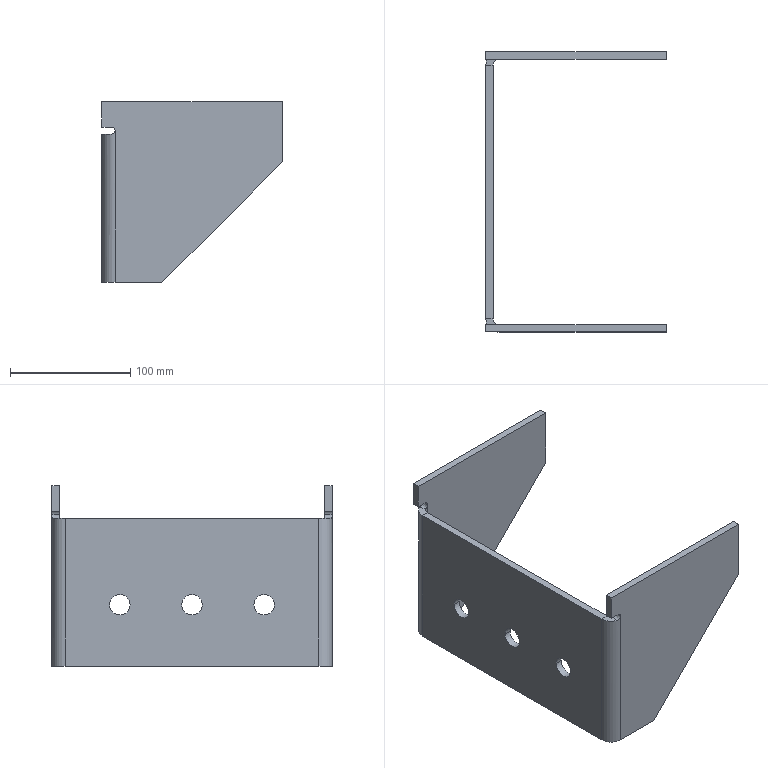Part | STEP file | SYL_0392D6J1SYL0380DJ100-148816 | 1 solid | 41 faces | box 150 x 233 x 150 mm | volume 363200 mm3 | plane 24 | cylinder 15 | spline 2 | commonest cylinder face diameters 17 x9 6 x2 10 x2 22 x2
STEP:
#1=CARTESIAN_POINT('',(6.,110.5,-90.5));
#2=VERTEX_POINT('',#1);
#3=CARTESIAN_POINT('',(6.,119.,-99.));
#4=VERTEX_POINT('',#3);
#5=CARTESIAN_POINT('',(6.,110.5,-99.));
#6=DIRECTION('',(-1.,0.,0.));
#7=DIRECTION('',(0.,-1.,0.));
#8=AXIS2_PLACEMENT_3D('',#5,#6,#7);
#9=CIRCLE('',#8,8.5);
#10=EDGE_CURVE('',#2,#4,#9,.T.);
#11=ORIENTED_EDGE('',*,*,#10,.F.);
#12=CARTESIAN_POINT('',(0.,110.5,-90.5));
#13=VERTEX_POINT('',#12);
#14=CARTESIAN_POINT('',(6.,110.5,-90.5));
#15=DIRECTION('',(-1.,0.,0.));
#16=VECTOR('',#15,1000.);
#17=LINE('',#14,#16);
#18=EDGE_CURVE('',#2,#13,#17,.T.);
#19=ORIENTED_EDGE('',*,*,#18,.T.);
#20=CARTESIAN_POINT('',(0.,119.,-99.));
#21=VERTEX_POINT('',#20);
#22=CARTESIAN_POINT('',(0.,110.5,-99.));
#23=DIRECTION('',(-1.,0.,0.));
#24=DIRECTION('',(0.,-1.,0.));
#25=AXIS2_PLACEMENT_3D('',#22,#23,#24);
#26=CIRCLE('',#25,8.5);
#27=EDGE_CURVE('',#13,#21,#26,.T.);
#28=ORIENTED_EDGE('',*,*,#27,.T.);
#29=CARTESIAN_POINT('',(6.,119.,-99.));
#30=DIRECTION('',(1.,0.,0.));
#31=VECTOR('',#30,1000.);
#32=LINE('',#29,#31);
#33=EDGE_CURVE('',#21,#4,#32,.T.);
#34=ORIENTED_EDGE('',*,*,#33,.T.);
#35=EDGE_LOOP('',(#11,#19,#28,#34));
#36=FACE_OUTER_BOUND('',#35,.T.);
#37=CARTESIAN_POINT('',(6.,110.5,-99.));
#38=DIRECTION('',(-1.,0.,0.));
#39=DIRECTION('',(0.,0.,1.));
#40=AXIS2_PLACEMENT_3D('',#37,#38,#39);
#41=CYLINDRICAL_SURFACE('',#40,8.5);
#42=ADVANCED_FACE('',(#36),#41,.F.);
#43=CARTESIAN_POINT('',(6.,170.5,-90.5));
#44=VERTEX_POINT('',#43);
#45=CARTESIAN_POINT('',(6.,179.,-99.));
#46=VERTEX_POINT('',#45);
#47=CARTESIAN_POINT('',(6.,170.5,-99.));
#48=DIRECTION('',(-1.,0.,0.));
#49=DIRECTION('',(0.,-1.,0.));
#50=AXIS2_PLACEMENT_3D('',#47,#48,#49);
#51=CIRCLE('',#50,8.5);
#52=EDGE_CURVE('',#44,#46,#51,.T.);
#53=ORIENTED_EDGE('',*,*,#52,.F.);
#54=CARTESIAN_POINT('',(0.,170.5,-90.5));
#55=VERTEX_POINT('',#54);
#56=CARTESIAN_POINT('',(6.,170.5,-90.5));
#57=DIRECTION('',(-1.,0.,0.));
#58=VECTOR('',#57,1000.);
#59=LINE('',#56,#58);
#60=EDGE_CURVE('',#44,#55,#59,.T.);
#61=ORIENTED_EDGE('',*,*,#60,.T.);
#62=CARTESIAN_POINT('',(0.,179.,-99.));
#63=VERTEX_POINT('',#62);
#64=CARTESIAN_POINT('',(0.,170.5,-99.));
#65=DIRECTION('',(-1.,0.,0.));
#66=DIRECTION('',(0.,-1.,0.));
#67=AXIS2_PLACEMENT_3D('',#64,#65,#66);
#68=CIRCLE('',#67,8.5);
#69=EDGE_CURVE('',#55,#63,#68,.T.);
#70=ORIENTED_EDGE('',*,*,#69,.T.);
#71=CARTESIAN_POINT('',(6.,179.,-99.));
#72=DIRECTION('',(1.,0.,0.));
#73=VECTOR('',#72,1000.);
#74=LINE('',#71,#73);
#75=EDGE_CURVE('',#63,#46,#74,.T.);
#76=ORIENTED_EDGE('',*,*,#75,.T.);
#77=EDGE_LOOP('',(#53,#61,#70,#76));
#78=FACE_OUTER_BOUND('',#77,.T.);
#79=CARTESIAN_POINT('',(6.,170.5,-99.));
#80=DIRECTION('',(-1.,0.,0.));
#81=DIRECTION('',(0.,0.,1.));
#82=AXIS2_PLACEMENT_3D('',#79,#80,#81);
#83=CYLINDRICAL_SURFACE('',#82,8.5);
#84=ADVANCED_FACE('',(#78),#83,.F.);
#85=CARTESIAN_POINT('',(6.,50.5,-90.5));
#86=VERTEX_POINT('',#85);
#87=CARTESIAN_POINT('',(6.,59.,-99.));
#88=VERTEX_POINT('',#87);
#89=CARTESIAN_POINT('',(6.,50.5,-99.));
#90=DIRECTION('',(-1.,0.,0.));
#91=DIRECTION('',(0.,-1.,0.));
#92=AXIS2_PLACEMENT_3D('',#89,#90,#91);
#93=CIRCLE('',#92,8.5);
#94=EDGE_CURVE('',#86,#88,#93,.T.);
#95=ORIENTED_EDGE('',*,*,#94,.F.);
#96=CARTESIAN_POINT('',(0.,50.5,-90.5));
#97=VERTEX_POINT('',#96);
#98=CARTESIAN_POINT('',(6.,50.5,-90.5));
#99=DIRECTION('',(-1.,0.,0.));
#100=VECTOR('',#99,1000.);
#101=LINE('',#98,#100);
#102=EDGE_CURVE('',#86,#97,#101,.T.);
#103=ORIENTED_EDGE('',*,*,#102,.T.);
#104=CARTESIAN_POINT('',(0.,59.,-99.));
#105=VERTEX_POINT('',#104);
#106=CARTESIAN_POINT('',(0.,50.5,-99.));
#107=DIRECTION('',(-1.,0.,0.));
#108=DIRECTION('',(0.,-1.,0.));
#109=AXIS2_PLACEMENT_3D('',#106,#107,#108);
#110=CIRCLE('',#109,8.5);
#111=EDGE_CURVE('',#97,#105,#110,.T.);
#112=ORIENTED_EDGE('',*,*,#111,.T.);
#113=CARTESIAN_POINT('',(6.,59.,-99.));
#114=DIRECTION('',(1.,0.,0.));
#115=VECTOR('',#114,1000.);
#116=LINE('',#113,#115);
#117=EDGE_CURVE('',#105,#88,#116,.T.);
#118=ORIENTED_EDGE('',*,*,#117,.T.);
#119=EDGE_LOOP('',(#95,#103,#112,#118));
#120=FACE_OUTER_BOUND('',#119,.T.);
#121=CARTESIAN_POINT('',(6.,50.5,-99.));
#122=DIRECTION('',(-1.,0.,0.));
#123=DIRECTION('',(0.,0.,1.));
#124=AXIS2_PLACEMENT_3D('',#121,#122,#123);
#125=CYLINDRICAL_SURFACE('',#124,8.5);
#126=ADVANCED_FACE('',(#120),#125,.F.);
#127=ORIENTED_EDGE('',*,*,#33,.F.);
#128=CARTESIAN_POINT('',(0.,102.,-99.));
#129=VERTEX_POINT('',#128);
#130=CARTESIAN_POINT('',(0.,110.5,-99.));
#131=DIRECTION('',(-1.,0.,0.));
#132=DIRECTION('',(0.,-1.,0.));
#133=AXIS2_PLACEMENT_3D('',#130,#131,#132);
#134=CIRCLE('',#133,8.5);
#135=EDGE_CURVE('',#21,#129,#134,.T.);
#136=ORIENTED_EDGE('',*,*,#135,.T.);
#137=CARTESIAN_POINT('',(6.,102.,-99.));
#138=VERTEX_POINT('',#137);
#139=CARTESIAN_POINT('',(6.,102.,-99.));
#140=DIRECTION('',(1.,0.,0.));
#141=VECTOR('',#140,1000.);
#142=LINE('',#139,#141);
#143=EDGE_CURVE('',#129,#138,#142,.T.);
#144=ORIENTED_EDGE('',*,*,#143,.T.);
#145=CARTESIAN_POINT('',(6.,110.5,-99.));
#146=DIRECTION('',(-1.,0.,0.));
#147=DIRECTION('',(0.,1.,0.));
#148=AXIS2_PLACEMENT_3D('',#145,#146,#147);
#149=CIRCLE('',#148,8.5);
#150=EDGE_CURVE('',#4,#138,#149,.T.);
#151=ORIENTED_EDGE('',*,*,#150,.F.);
#152=EDGE_LOOP('',(#127,#136,#144,#151));
#153=FACE_OUTER_BOUND('',#152,.T.);
#154=CARTESIAN_POINT('',(6.,110.5,-99.));
#155=DIRECTION('',(-1.,0.,0.));
#156=DIRECTION('',(0.,0.,1.));
#157=AXIS2_PLACEMENT_3D('',#154,#155,#156);
#158=CYLINDRICAL_SURFACE('',#157,8.5);
#159=ADVANCED_FACE('',(#153),#158,.F.);
#160=ORIENTED_EDGE('',*,*,#75,.F.);
#161=CARTESIAN_POINT('',(0.,162.,-99.));
#162=VERTEX_POINT('',#161);
#163=CARTESIAN_POINT('',(0.,170.5,-99.));
#164=DIRECTION('',(-1.,0.,0.));
#165=DIRECTION('',(0.,-1.,0.));
#166=AXIS2_PLACEMENT_3D('',#163,#164,#165);
#167=CIRCLE('',#166,8.5);
#168=EDGE_CURVE('',#63,#162,#167,.T.);
#169=ORIENTED_EDGE('',*,*,#168,.T.);
#170=CARTESIAN_POINT('',(6.,162.,-99.));
#171=VERTEX_POINT('',#170);
#172=CARTESIAN_POINT('',(6.,162.,-99.));
#173=DIRECTION('',(1.,0.,0.));
#174=VECTOR('',#173,1000.);
#175=LINE('',#172,#174);
#176=EDGE_CURVE('',#162,#171,#175,.T.);
#177=ORIENTED_EDGE('',*,*,#176,.T.);
#178=CARTESIAN_POINT('',(6.,170.5,-99.));
#179=DIRECTION('',(-1.,0.,0.));
#180=DIRECTION('',(0.,1.,0.));
#181=AXIS2_PLACEMENT_3D('',#178,#179,#180);
#182=CIRCLE('',#181,8.5);
#183=EDGE_CURVE('',#46,#171,#182,.T.);
#184=ORIENTED_EDGE('',*,*,#183,.F.);
#185=EDGE_LOOP('',(#160,#169,#177,#184));
#186=FACE_OUTER_BOUND('',#185,.T.);
#187=CARTESIAN_POINT('',(6.,170.5,-99.));
#188=DIRECTION('',(-1.,0.,0.));
#189=DIRECTION('',(0.,0.,1.));
#190=AXIS2_PLACEMENT_3D('',#187,#188,#189);
#191=CYLINDRICAL_SURFACE('',#190,8.5);
#192=ADVANCED_FACE('',(#186),#191,.F.);
#193=ORIENTED_EDGE('',*,*,#117,.F.);
#194=CARTESIAN_POINT('',(0.,42.,-99.));
#195=VERTEX_POINT('',#194);
#196=CARTESIAN_POINT('',(0.,50.5,-99.));
#197=DIRECTION('',(-1.,0.,0.));
#198=DIRECTION('',(0.,-1.,0.));
#199=AXIS2_PLACEMENT_3D('',#196,#197,#198);
#200=CIRCLE('',#199,8.5);
#201=EDGE_CURVE('',#105,#195,#200,.T.);
#202=ORIENTED_EDGE('',*,*,#201,.T.);
#203=CARTESIAN_POINT('',(6.,42.,-99.));
#204=VERTEX_POINT('',#203);
#205=CARTESIAN_POINT('',(6.,42.,-99.));
#206=DIRECTION('',(1.,0.,0.));
#207=VECTOR('',#206,1000.);
#208=LINE('',#205,#207);
#209=EDGE_CURVE('',#195,#204,#208,.T.);
#210=ORIENTED_EDGE('',*,*,#209,.T.);
#211=CARTESIAN_POINT('',(6.,50.5,-99.));
#212=DIRECTION('',(-1.,0.,0.));
#213=DIRECTION('',(0.,1.,0.));
#214=AXIS2_PLACEMENT_3D('',#211,#212,#213);
#215=CIRCLE('',#214,8.5);
#216=EDGE_CURVE('',#88,#204,#215,.T.);
#217=ORIENTED_EDGE('',*,*,#216,.F.);
#218=EDGE_LOOP('',(#193,#202,#210,#217));
#219=FACE_OUTER_BOUND('',#218,.T.);
#220=CARTESIAN_POINT('',(6.,50.5,-99.));
#221=DIRECTION('',(-1.,0.,0.));
#222=DIRECTION('',(0.,0.,1.));
#223=AXIS2_PLACEMENT_3D('',#220,#221,#222);
#224=CYLINDRICAL_SURFACE('',#223,8.5);
#225=ADVANCED_FACE('',(#219),#224,.F.);
#226=CARTESIAN_POINT('',(11.,-6.,-24.));
#227=VERTEX_POINT('',#226);
#228=CARTESIAN_POINT('',(11.,0.,-24.));
#229=VERTEX_POINT('',#228);
#230=CARTESIAN_POINT('',(11.,-6.,-24.));
#231=CARTESIAN_POINT('',(11.,0.,-24.));
#232=B_SPLINE_CURVE_WITH_KNOTS('',1,(#230,#231),.UNSPECIFIED.,.F.,.F.,(2,2),(0.,1.),.UNSPECIFIED.);
#233=EDGE_CURVE('',#227,#229,#232,.T.);
#234=ORIENTED_EDGE('',*,*,#233,.F.);
#235=CARTESIAN_POINT('',(8.,-6.,-21.));
#236=VERTEX_POINT('',#235);
#237=CARTESIAN_POINT('',(8.,-6.,-24.));
#238=DIRECTION('',(0.,-1.,0.));
#239=DIRECTION('',(0.,0.,-1.));
#240=AXIS2_PLACEMENT_3D('',#237,#238,#239);
#241=CIRCLE('',#240,3.);
#242=EDGE_CURVE('',#227,#236,#241,.T.);
#243=ORIENTED_EDGE('',*,*,#242,.T.);
#244=CARTESIAN_POINT('',(8.,0.,-21.));
#245=VERTEX_POINT('',#244);
#246=CARTESIAN_POINT('',(8.,0.,-21.));
#247=DIRECTION('',(0.,1.,0.));
#248=VECTOR('',#247,1000.);
#249=LINE('',#246,#248);
#250=EDGE_CURVE('',#236,#245,#249,.T.);
#251=ORIENTED_EDGE('',*,*,#250,.T.);
#252=CARTESIAN_POINT('',(8.,0.,-24.));
#253=DIRECTION('',(0.,-1.,0.));
#254=DIRECTION('',(1.,0.,0.));
#255=AXIS2_PLACEMENT_3D('',#252,#253,#254);
#256=CIRCLE('',#255,3.);
#257=EDGE_CURVE('',#229,#245,#256,.T.);
#258=ORIENTED_EDGE('',*,*,#257,.F.);
#259=EDGE_LOOP('',(#234,#243,#251,#258));
#260=FACE_OUTER_BOUND('',#259,.T.);
#261=CARTESIAN_POINT('',(8.,0.,-24.));
#262=DIRECTION('',(0.,1.,0.));
#263=DIRECTION('',(0.,0.,1.));
#264=AXIS2_PLACEMENT_3D('',#261,#262,#263);
#265=CYLINDRICAL_SURFACE('',#264,3.);
#266=ADVANCED_FACE('',(#260),#265,.F.);
#267=ORIENTED_EDGE('',*,*,#250,.F.);
#268=CARTESIAN_POINT('',(0.,-6.,-21.));
#269=VERTEX_POINT('',#268);
#270=CARTESIAN_POINT('',(0.,-6.,-21.));
#271=DIRECTION('',(-1.,0.,0.));
#272=VECTOR('',#271,1000.);
#273=LINE('',#270,#272);
#274=EDGE_CURVE('',#236,#269,#273,.T.);
#275=ORIENTED_EDGE('',*,*,#274,.T.);
#276=CARTESIAN_POINT('',(0.,0.,-21.));
#277=VERTEX_POINT('',#276);
#278=CARTESIAN_POINT('',(0.,0.,-21.));
#279=DIRECTION('',(0.,1.,0.));
#280=VECTOR('',#279,1000.);
#281=LINE('',#278,#280);
#282=EDGE_CURVE('',#269,#277,#281,.T.);
#283=ORIENTED_EDGE('',*,*,#282,.T.);
#284=CARTESIAN_POINT('',(8.,0.,-21.));
#285=DIRECTION('',(-1.,0.,0.));
#286=VECTOR('',#285,1000.);
#287=LINE('',#284,#286);
#288=EDGE_CURVE('',#245,#277,#287,.T.);
#289=ORIENTED_EDGE('',*,*,#288,.F.);
#290=EDGE_LOOP('',(#267,#275,#283,#289));
#291=FACE_OUTER_BOUND('',#290,.T.);
#292=CARTESIAN_POINT('',(8.,0.,-21.));
#293=DIRECTION('',(0.,0.,-1.));
#294=DIRECTION('',(-1.,0.,0.));
#295=AXIS2_PLACEMENT_3D('',#292,#293,#294);
#296=PLANE('',#295);
#297=ADVANCED_FACE('',(#291),#296,.T.);
#298=ORIENTED_EDGE('',*,*,#282,.F.);
#299=CARTESIAN_POINT('',(0.,-6.,0.));
#300=VERTEX_POINT('',#299);
#301=CARTESIAN_POINT('',(0.,-6.,0.));
#302=DIRECTION('',(0.,0.,1.));
#303=VECTOR('',#302,1000.);
#304=LINE('',#301,#303);
#305=EDGE_CURVE('',#269,#300,#304,.T.);
#306=ORIENTED_EDGE('',*,*,#305,.T.);
#307=CARTESIAN_POINT('',(0.,0.,0.));
#308=VERTEX_POINT('',#307);
#309=CARTESIAN_POINT('',(0.,0.,0.));
#310=DIRECTION('',(0.,1.,0.));
#311=VECTOR('',#310,1000.);
#312=LINE('',#309,#311);
#313=EDGE_CURVE('',#300,#308,#312,.T.);
#314=ORIENTED_EDGE('',*,*,#313,.T.);
#315=CARTESIAN_POINT('',(0.,0.,-21.));
#316=DIRECTION('',(0.,0.,1.));
#317=VECTOR('',#316,1000.);
#318=LINE('',#315,#317);
#319=EDGE_CURVE('',#277,#308,#318,.T.);
#320=ORIENTED_EDGE('',*,*,#319,.F.);
#321=EDGE_LOOP('',(#298,#306,#314,#320));
#322=FACE_OUTER_BOUND('',#321,.T.);
#323=CARTESIAN_POINT('',(0.,0.,-21.));
#324=DIRECTION('',(-1.,0.,0.));
#325=DIRECTION('',(0.,0.,1.));
#326=AXIS2_PLACEMENT_3D('',#323,#324,#325);
#327=PLANE('',#326);
#328=ADVANCED_FACE('',(#322),#327,.T.);
#329=ORIENTED_EDGE('',*,*,#313,.F.);
#330=CARTESIAN_POINT('',(150.,-6.,0.));
#331=VERTEX_POINT('',#330);
#332=CARTESIAN_POINT('',(0.,-6.,0.));
#333=DIRECTION('',(1.,0.,0.));
#334=VECTOR('',#333,1000.);
#335=LINE('',#332,#334);
#336=EDGE_CURVE('',#300,#331,#335,.T.);
#337=ORIENTED_EDGE('',*,*,#336,.T.);
#338=CARTESIAN_POINT('',(150.,0.,0.));
#339=VERTEX_POINT('',#338);
#340=CARTESIAN_POINT('',(150.,0.,0.));
#341=DIRECTION('',(0.,1.,0.));
#342=VECTOR('',#341,1000.);
#343=LINE('',#340,#342);
#344=EDGE_CURVE('',#331,#339,#343,.T.);
#345=ORIENTED_EDGE('',*,*,#344,.T.);
#346=CARTESIAN_POINT('',(0.,0.,0.));
#347=DIRECTION('',(1.,0.,0.));
#348=VECTOR('',#347,1000.);
#349=LINE('',#346,#348);
#350=EDGE_CURVE('',#308,#339,#349,.T.);
#351=ORIENTED_EDGE('',*,*,#350,.F.);
#352=EDGE_LOOP('',(#329,#337,#345,#351));
#353=FACE_OUTER_BOUND('',#352,.T.);
#354=CARTESIAN_POINT('',(0.,0.,0.));
#355=DIRECTION('',(0.,0.,1.));
#356=DIRECTION('',(1.,0.,0.));
#357=AXIS2_PLACEMENT_3D('',#354,#355,#356);
#358=PLANE('',#357);
#359=ADVANCED_FACE('',(#353),#358,.T.);
#360=ORIENTED_EDGE('',*,*,#344,.F.);
#361=CARTESIAN_POINT('',(150.,-6.,-50.));
#362=VERTEX_POINT('',#361);
#363=CARTESIAN_POINT('',(150.,-6.,0.));
#364=DIRECTION('',(0.,0.,-1.));
#365=VECTOR('',#364,1000.);
#366=LINE('',#363,#365);
#367=EDGE_CURVE('',#331,#362,#366,.T.);
#368=ORIENTED_EDGE('',*,*,#367,.T.);
#369=CARTESIAN_POINT('',(150.,0.,-50.));
#370=VERTEX_POINT('',#369);
#371=CARTESIAN_POINT('',(150.,0.,-50.));
#372=DIRECTION('',(0.,1.,0.));
#373=VECTOR('',#372,1000.);
#374=LINE('',#371,#373);
#375=EDGE_CURVE('',#362,#370,#374,.T.);
#376=ORIENTED_EDGE('',*,*,#375,.T.);
#377=CARTESIAN_POINT('',(150.,0.,0.));
#378=DIRECTION('',(0.,0.,-1.));
#379=VECTOR('',#378,1000.);
#380=LINE('',#377,#379);
#381=EDGE_CURVE('',#339,#370,#380,.T.);
#382=ORIENTED_EDGE('',*,*,#381,.F.);
#383=EDGE_LOOP('',(#360,#368,#376,#382));
#384=FACE_OUTER_BOUND('',#383,.T.);
#385=CARTESIAN_POINT('',(150.,0.,0.));
#386=DIRECTION('',(1.,0.,0.));
#387=DIRECTION('',(0.,0.,-1.));
#388=AXIS2_PLACEMENT_3D('',#385,#386,#387);
#389=PLANE('',#388);
#390=ADVANCED_FACE('',(#384),#389,.T.);
#391=ORIENTED_EDGE('',*,*,#375,.F.);
#392=CARTESIAN_POINT('',(50.,-6.,-150.));
#393=VERTEX_POINT('',#392);
#394=CARTESIAN_POINT('',(150.,-6.,-50.));
#395=DIRECTION('',(-0.7071,0.,-0.7071));
#396=VECTOR('',#395,1000.);
#397=LINE('',#394,#396);
#398=EDGE_CURVE('',#362,#393,#397,.T.);
#399=ORIENTED_EDGE('',*,*,#398,.T.);
#400=CARTESIAN_POINT('',(50.,0.,-150.));
#401=VERTEX_POINT('',#400);
#402=CARTESIAN_POINT('',(50.,0.,-150.));
#403=DIRECTION('',(0.,1.,0.));
#404=VECTOR('',#403,1000.);
#405=LINE('',#402,#404);
#406=EDGE_CURVE('',#393,#401,#405,.T.);
#407=ORIENTED_EDGE('',*,*,#406,.T.);
#408=CARTESIAN_POINT('',(150.,0.,-50.));
#409=DIRECTION('',(-0.7071,0.,-0.7071));
#410=VECTOR('',#409,1000.);
#411=LINE('',#408,#410);
#412=EDGE_CURVE('',#370,#401,#411,.T.);
#413=ORIENTED_EDGE('',*,*,#412,.F.);
#414=EDGE_LOOP('',(#391,#399,#407,#413));
#415=FACE_OUTER_BOUND('',#414,.T.);
#416=CARTESIAN_POINT('',(150.,0.,-50.));
#417=DIRECTION('',(0.7071,0.,-0.7071));
#418=DIRECTION('',(-0.7071,0.,-0.7071));
#419=AXIS2_PLACEMENT_3D('',#416,#417,#418);
#420=PLANE('',#419);
#421=ADVANCED_FACE('',(#415),#420,.T.);
#422=ORIENTED_EDGE('',*,*,#406,.F.);
#423=CARTESIAN_POINT('',(11.,-6.,-150.));
#424=VERTEX_POINT('',#423);
#425=CARTESIAN_POINT('',(0.,-6.,-150.));
#426=DIRECTION('',(-1.,0.,0.));
#427=VECTOR('',#426,1000.);
#428=LINE('',#425,#427);
#429=EDGE_CURVE('',#393,#424,#428,.T.);
#430=ORIENTED_EDGE('',*,*,#429,.T.);
#431=CARTESIAN_POINT('',(11.,0.,-150.));
#432=VERTEX_POINT('',#431);
#433=CARTESIAN_POINT('',(11.,0.,-150.));
#434=DIRECTION('',(0.,1.,0.));
#435=VECTOR('',#434,1000.);
#436=LINE('',#433,#435);
#437=EDGE_CURVE('',#424,#432,#436,.T.);
#438=ORIENTED_EDGE('',*,*,#437,.T.);
#439=CARTESIAN_POINT('',(50.,0.,-150.));
#440=DIRECTION('',(-1.,0.,0.));
#441=VECTOR('',#440,1000.);
#442=LINE('',#439,#441);
#443=EDGE_CURVE('',#401,#432,#442,.T.);
#444=ORIENTED_EDGE('',*,*,#443,.F.);
#445=EDGE_LOOP('',(#422,#430,#438,#444));
#446=FACE_OUTER_BOUND('',#445,.T.);
#447=CARTESIAN_POINT('',(50.,0.,-150.));
#448=DIRECTION('',(0.,0.,-1.));
#449=DIRECTION('',(-1.,0.,0.));
#450=AXIS2_PLACEMENT_3D('',#447,#448,#449);
#451=PLANE('',#450);
#452=ADVANCED_FACE('',(#446),#451,.T.);
#453=ORIENTED_EDGE('',*,*,#437,.F.);
#454=CARTESIAN_POINT('',(0.,5.,-150.));
#455=VERTEX_POINT('',#454);
#456=CARTESIAN_POINT('',(11.,5.,-150.));
#457=DIRECTION('',(0.,0.,1.));
#458=DIRECTION('',(1.,0.,0.));
#459=AXIS2_PLACEMENT_3D('',#456,#457,#458);
#460=CIRCLE('',#459,11.);
#461=EDGE_CURVE('',#455,#424,#460,.T.);
#462=ORIENTED_EDGE('',*,*,#461,.F.);
#463=CARTESIAN_POINT('',(6.,5.,-150.));
#464=VERTEX_POINT('',#463);
#465=CARTESIAN_POINT('',(6.,5.,-150.));
#466=DIRECTION('',(1.,0.,0.));
#467=VECTOR('',#466,1000.);
#468=LINE('',#465,#467);
#469=EDGE_CURVE('',#455,#464,#468,.T.);
#470=ORIENTED_EDGE('',*,*,#469,.T.);
#471=CARTESIAN_POINT('',(11.,5.,-150.));
#472=DIRECTION('',(0.,0.,1.));
#473=DIRECTION('',(-1.,0.,0.));
#474=AXIS2_PLACEMENT_3D('',#471,#472,#473);
#475=CIRCLE('',#474,5.);
#476=EDGE_CURVE('',#464,#432,#475,.T.);
#477=ORIENTED_EDGE('',*,*,#476,.T.);
#478=EDGE_LOOP('',(#453,#462,#470,#477));
#479=FACE_OUTER_BOUND('',#478,.T.);
#480=CARTESIAN_POINT('',(11.,5.,-150.));
#481=DIRECTION('',(0.,0.,-1.));
#482=DIRECTION('',(-1.,0.,0.));
#483=AXIS2_PLACEMENT_3D('',#480,#481,#482);
#484=PLANE('',#483);
#485=ADVANCED_FACE('',(#479),#484,.T.);
#486=ORIENTED_EDGE('',*,*,#469,.F.);
#487=CARTESIAN_POINT('',(0.,216.,-150.));
#488=VERTEX_POINT('',#487);
#489=CARTESIAN_POINT('',(0.,-6.,-150.));
#490=DIRECTION('',(0.,1.,0.));
#491=VECTOR('',#490,1000.);
#492=LINE('',#489,#491);
#493=EDGE_CURVE('',#455,#488,#492,.T.);
#494=ORIENTED_EDGE('',*,*,#493,.T.);
#495=CARTESIAN_POINT('',(6.,216.,-150.));
#496=VERTEX_POINT('',#495);
#497=CARTESIAN_POINT('',(6.,216.,-150.));
#498=DIRECTION('',(1.,0.,0.));
#499=VECTOR('',#498,1000.);
#500=LINE('',#497,#499);
#501=EDGE_CURVE('',#488,#496,#500,.T.);
#502=ORIENTED_EDGE('',*,*,#501,.T.);
#503=CARTESIAN_POINT('',(6.,5.,-150.));
#504=DIRECTION('',(0.,1.,0.));
#505=VECTOR('',#504,1000.);
#506=LINE('',#503,#505);
#507=EDGE_CURVE('',#464,#496,#506,.T.);
#508=ORIENTED_EDGE('',*,*,#507,.F.);
#509=EDGE_LOOP('',(#486,#494,#502,#508));
#510=FACE_OUTER_BOUND('',#509,.T.);
#511=CARTESIAN_POINT('',(6.,5.,-150.));
#512=DIRECTION('',(0.,0.,1.));
#513=DIRECTION('',(0.,1.,0.));
#514=AXIS2_PLACEMENT_3D('',#511,#512,#513);
#515=PLANE('',#514);
#516=ADVANCED_FACE('',(#510),#515,.F.);
#517=ORIENTED_EDGE('',*,*,#501,.F.);
#518=CARTESIAN_POINT('',(11.,227.,-150.));
#519=VERTEX_POINT('',#518);
#520=CARTESIAN_POINT('',(11.,216.,-150.));
#521=DIRECTION('',(0.,0.,1.));
#522=DIRECTION('',(-1.,0.,0.));
#523=AXIS2_PLACEMENT_3D('',#520,#521,#522);
#524=CIRCLE('',#523,11.);
#525=EDGE_CURVE('',#519,#488,#524,.T.);
#526=ORIENTED_EDGE('',*,*,#525,.F.);
#527=CARTESIAN_POINT('',(11.,221.,-150.));
#528=VERTEX_POINT('',#527);
#529=CARTESIAN_POINT('',(11.,221.,-150.));
#530=DIRECTION('',(0.,-1.,0.));
#531=VECTOR('',#530,1000.);
#532=LINE('',#529,#531);
#533=EDGE_CURVE('',#519,#528,#532,.T.);
#534=ORIENTED_EDGE('',*,*,#533,.T.);
#535=CARTESIAN_POINT('',(11.,216.,-150.));
#536=DIRECTION('',(0.,0.,1.));
#537=DIRECTION('',(0.,1.,0.));
#538=AXIS2_PLACEMENT_3D('',#535,#536,#537);
#539=CIRCLE('',#538,5.);
#540=EDGE_CURVE('',#528,#496,#539,.T.);
#541=ORIENTED_EDGE('',*,*,#540,.T.);
#542=EDGE_LOOP('',(#517,#526,#534,#541));
#543=FACE_OUTER_BOUND('',#542,.T.);
#544=CARTESIAN_POINT('',(11.,216.,-150.));
#545=DIRECTION('',(0.,0.,-1.));
#546=DIRECTION('',(-1.,0.,0.));
#547=AXIS2_PLACEMENT_3D('',#544,#545,#546);
#548=PLANE('',#547);
#549=ADVANCED_FACE('',(#543),#548,.T.);
#550=ORIENTED_EDGE('',*,*,#533,.F.);
#551=CARTESIAN_POINT('',(50.,227.,-150.));
#552=VERTEX_POINT('',#551);
#553=CARTESIAN_POINT('',(0.,227.,-150.));
#554=DIRECTION('',(-1.,0.,0.));
#555=VECTOR('',#554,1000.);
#556=LINE('',#553,#555);
#557=EDGE_CURVE('',#552,#519,#556,.T.);
#558=ORIENTED_EDGE('',*,*,#557,.F.);
#559=CARTESIAN_POINT('',(50.,221.,-150.));
#560=VERTEX_POINT('',#559);
#561=CARTESIAN_POINT('',(50.,221.,-150.));
#562=DIRECTION('',(0.,-1.,0.));
#563=VECTOR('',#562,1000.);
#564=LINE('',#561,#563);
#565=EDGE_CURVE('',#552,#560,#564,.T.);
#566=ORIENTED_EDGE('',*,*,#565,.T.);
#567=CARTESIAN_POINT('',(50.,221.,-150.));
#568=DIRECTION('',(-1.,0.,0.));
#569=VECTOR('',#568,1000.);
#570=LINE('',#567,#569);
#571=EDGE_CURVE('',#560,#528,#570,.T.);
#572=ORIENTED_EDGE('',*,*,#571,.T.);
#573=EDGE_LOOP('',(#550,#558,#566,#572));
#574=FACE_OUTER_BOUND('',#573,.T.);
#575=CARTESIAN_POINT('',(50.,221.,-150.));
#576=DIRECTION('',(0.,0.,-1.));
#577=DIRECTION('',(-1.,0.,0.));
#578=AXIS2_PLACEMENT_3D('',#575,#576,#577);
#579=PLANE('',#578);
#580=ADVANCED_FACE('',(#574),#579,.T.);
#581=ORIENTED_EDGE('',*,*,#565,.F.);
#582=CARTESIAN_POINT('',(150.,227.,-50.));
#583=VERTEX_POINT('',#582);
#584=CARTESIAN_POINT('',(50.,227.,-150.));
#585=DIRECTION('',(0.7071,0.,0.7071));
#586=VECTOR('',#585,1000.);
#587=LINE('',#584,#586);
#588=EDGE_CURVE('',#552,#583,#587,.T.);
#589=ORIENTED_EDGE('',*,*,#588,.T.);
#590=CARTESIAN_POINT('',(150.,221.,-50.));
#591=VERTEX_POINT('',#590);
#592=CARTESIAN_POINT('',(150.,221.,-50.));
#593=DIRECTION('',(0.,-1.,0.));
#594=VECTOR('',#593,1000.);
#595=LINE('',#592,#594);
#596=EDGE_CURVE('',#583,#591,#595,.T.);
#597=ORIENTED_EDGE('',*,*,#596,.T.);
#598=CARTESIAN_POINT('',(50.,221.,-150.));
#599=DIRECTION('',(0.7071,0.,0.7071));
#600=VECTOR('',#599,1000.);
#601=LINE('',#598,#600);
#602=EDGE_CURVE('',#560,#591,#601,.T.);
#603=ORIENTED_EDGE('',*,*,#602,.F.);
#604=EDGE_LOOP('',(#581,#589,#597,#603));
#605=FACE_OUTER_BOUND('',#604,.T.);
#606=CARTESIAN_POINT('',(50.,221.,-150.));
#607=DIRECTION('',(-0.7071,0.,0.7071));
#608=DIRECTION('',(0.7071,0.,0.7071));
#609=AXIS2_PLACEMENT_3D('',#606,#607,#608);
#610=PLANE('',#609);
#611=ADVANCED_FACE('',(#605),#610,.F.);
#612=ORIENTED_EDGE('',*,*,#596,.F.);
#613=CARTESIAN_POINT('',(150.,227.,0.));
#614=VERTEX_POINT('',#613);
#615=CARTESIAN_POINT('',(150.,227.,0.));
#616=DIRECTION('',(0.,0.,-1.));
#617=VECTOR('',#616,1000.);
#618=LINE('',#615,#617);
#619=EDGE_CURVE('',#614,#583,#618,.T.);
#620=ORIENTED_EDGE('',*,*,#619,.F.);
#621=CARTESIAN_POINT('',(150.,221.,0.));
#622=VERTEX_POINT('',#621);
#623=CARTESIAN_POINT('',(150.,221.,0.));
#624=DIRECTION('',(0.,-1.,0.));
#625=VECTOR('',#624,1000.);
#626=LINE('',#623,#625);
#627=EDGE_CURVE('',#614,#622,#626,.T.);
#628=ORIENTED_EDGE('',*,*,#627,.T.);
#629=CARTESIAN_POINT('',(150.,221.,0.));
#630=DIRECTION('',(0.,0.,-1.));
#631=VECTOR('',#630,1000.);
#632=LINE('',#629,#631);
#633=EDGE_CURVE('',#622,#591,#632,.T.);
#634=ORIENTED_EDGE('',*,*,#633,.T.);
#635=EDGE_LOOP('',(#612,#620,#628,#634));
#636=FACE_OUTER_BOUND('',#635,.T.);
#637=CARTESIAN_POINT('',(150.,221.,0.));
#638=DIRECTION('',(1.,0.,0.));
#639=DIRECTION('',(0.,0.,-1.));
#640=AXIS2_PLACEMENT_3D('',#637,#638,#639);
#641=PLANE('',#640);
#642=ADVANCED_FACE('',(#636),#641,.T.);
#643=ORIENTED_EDGE('',*,*,#627,.F.);
#644=CARTESIAN_POINT('',(0.,227.,0.));
#645=VERTEX_POINT('',#644);
#646=CARTESIAN_POINT('',(0.,227.,0.));
#647=DIRECTION('',(1.,0.,0.));
#648=VECTOR('',#647,1000.);
#649=LINE('',#646,#648);
#650=EDGE_CURVE('',#645,#614,#649,.T.);
#651=ORIENTED_EDGE('',*,*,#650,.F.);
#652=CARTESIAN_POINT('',(0.,221.,0.));
#653=VERTEX_POINT('',#652);
#654=CARTESIAN_POINT('',(0.,221.,0.));
#655=DIRECTION('',(0.,-1.,0.));
#656=VECTOR('',#655,1000.);
#657=LINE('',#654,#656);
#658=EDGE_CURVE('',#645,#653,#657,.T.);
#659=ORIENTED_EDGE('',*,*,#658,.T.);
#660=CARTESIAN_POINT('',(0.,221.,0.));
#661=DIRECTION('',(1.,0.,0.));
#662=VECTOR('',#661,1000.);
#663=LINE('',#660,#662);
#664=EDGE_CURVE('',#653,#622,#663,.T.);
#665=ORIENTED_EDGE('',*,*,#664,.T.);
#666=EDGE_LOOP('',(#643,#651,#659,#665));
#667=FACE_OUTER_BOUND('',#666,.T.);
#668=CARTESIAN_POINT('',(0.,221.,0.));
#669=DIRECTION('',(0.,0.,1.));
#670=DIRECTION('',(1.,0.,0.));
#671=AXIS2_PLACEMENT_3D('',#668,#669,#670);
#672=PLANE('',#671);
#673=ADVANCED_FACE('',(#667),#672,.T.);
#674=ORIENTED_EDGE('',*,*,#658,.F.);
#675=CARTESIAN_POINT('',(0.,227.,-21.));
#676=VERTEX_POINT('',#675);
#677=CARTESIAN_POINT('',(0.,227.,0.));
#678=DIRECTION('',(0.,0.,1.));
#679=VECTOR('',#678,1000.);
#680=LINE('',#677,#679);
#681=EDGE_CURVE('',#676,#645,#680,.T.);
#682=ORIENTED_EDGE('',*,*,#681,.F.);
#683=CARTESIAN_POINT('',(0.,221.,-21.));
#684=VERTEX_POINT('',#683);
#685=CARTESIAN_POINT('',(0.,221.,-21.));
#686=DIRECTION('',(0.,-1.,0.));
#687=VECTOR('',#686,1000.);
#688=LINE('',#685,#687);
#689=EDGE_CURVE('',#676,#684,#688,.T.);
#690=ORIENTED_EDGE('',*,*,#689,.T.);
#691=CARTESIAN_POINT('',(0.,221.,-21.));
#692=DIRECTION('',(0.,0.,1.));
#693=VECTOR('',#692,1000.);
#694=LINE('',#691,#693);
#695=EDGE_CURVE('',#684,#653,#694,.T.);
#696=ORIENTED_EDGE('',*,*,#695,.T.);
#697=EDGE_LOOP('',(#674,#682,#690,#696));
#698=FACE_OUTER_BOUND('',#697,.T.);
#699=CARTESIAN_POINT('',(0.,221.,-21.));
#700=DIRECTION('',(-1.,0.,0.));
#701=DIRECTION('',(0.,0.,1.));
#702=AXIS2_PLACEMENT_3D('',#699,#700,#701);
#703=PLANE('',#702);
#704=ADVANCED_FACE('',(#698),#703,.T.);
#705=ORIENTED_EDGE('',*,*,#689,.F.);
#706=CARTESIAN_POINT('',(8.,227.,-21.));
#707=VERTEX_POINT('',#706);
#708=CARTESIAN_POINT('',(0.,227.,-21.));
#709=DIRECTION('',(-1.,0.,0.));
#710=VECTOR('',#709,1000.);
#711=LINE('',#708,#710);
#712=EDGE_CURVE('',#707,#676,#711,.T.);
#713=ORIENTED_EDGE('',*,*,#712,.F.);
#714=CARTESIAN_POINT('',(8.,221.,-21.));
#715=VERTEX_POINT('',#714);
#716=CARTESIAN_POINT('',(8.,221.,-21.));
#717=DIRECTION('',(0.,-1.,0.));
#718=VECTOR('',#717,1000.);
#719=LINE('',#716,#718);
#720=EDGE_CURVE('',#707,#715,#719,.T.);
#721=ORIENTED_EDGE('',*,*,#720,.T.);
#722=CARTESIAN_POINT('',(8.,221.,-21.));
#723=DIRECTION('',(-1.,0.,0.));
#724=VECTOR('',#723,1000.);
#725=LINE('',#722,#724);
#726=EDGE_CURVE('',#715,#684,#725,.T.);
#727=ORIENTED_EDGE('',*,*,#726,.T.);
#728=EDGE_LOOP('',(#705,#713,#721,#727));
#729=FACE_OUTER_BOUND('',#728,.T.);
#730=CARTESIAN_POINT('',(8.,221.,-21.));
#731=DIRECTION('',(0.,0.,-1.));
#732=DIRECTION('',(-1.,0.,0.));
#733=AXIS2_PLACEMENT_3D('',#730,#731,#732);
#734=PLANE('',#733);
#735=ADVANCED_FACE('',(#729),#734,.T.);
#736=ORIENTED_EDGE('',*,*,#720,.F.);
#737=CARTESIAN_POINT('',(11.,227.,-24.));
#738=VERTEX_POINT('',#737);
#739=CARTESIAN_POINT('',(8.,227.,-24.));
#740=DIRECTION('',(0.,1.,0.));
#741=DIRECTION('',(-1.,0.,0.));
#742=AXIS2_PLACEMENT_3D('',#739,#740,#741);
#743=CIRCLE('',#742,3.);
#744=EDGE_CURVE('',#707,#738,#743,.T.);
#745=ORIENTED_EDGE('',*,*,#744,.T.);
#746=CARTESIAN_POINT('',(11.,221.,-24.));
#747=VERTEX_POINT('',#746);
#748=CARTESIAN_POINT('',(11.,227.,-24.));
#749=CARTESIAN_POINT('',(11.,225.,-24.));
#750=CARTESIAN_POINT('',(11.,223.,-24.));
#751=CARTESIAN_POINT('',(11.,221.,-24.));
#752=B_SPLINE_CURVE_WITH_KNOTS('',3,(#748,#749,#750,#751),.UNSPECIFIED.,.F.,.F.,(4,4),(0.,1.),.UNSPECIFIED.);
#753=EDGE_CURVE('',#738,#747,#752,.T.);
#754=ORIENTED_EDGE('',*,*,#753,.T.);
#755=CARTESIAN_POINT('',(8.,221.,-24.));
#756=DIRECTION('',(0.,1.,0.));
#757=DIRECTION('',(0.,0.,1.));
#758=AXIS2_PLACEMENT_3D('',#755,#756,#757);
#759=CIRCLE('',#758,3.);
#760=EDGE_CURVE('',#715,#747,#759,.T.);
#761=ORIENTED_EDGE('',*,*,#760,.F.);
#762=EDGE_LOOP('',(#736,#745,#754,#761));
#763=FACE_OUTER_BOUND('',#762,.T.);
#764=CARTESIAN_POINT('',(8.,221.,-24.));
#765=DIRECTION('',(0.,1.,0.));
#766=DIRECTION('',(-1.,0.,0.));
#767=AXIS2_PLACEMENT_3D('',#764,#765,#766);
#768=CYLINDRICAL_SURFACE('',#767,3.);
#769=ADVANCED_FACE('',(#763),#768,.F.);
#770=ORIENTED_EDGE('',*,*,#753,.F.);
#771=CARTESIAN_POINT('',(6.692,226.121,-27.));
#772=VERTEX_POINT('',#771);
#773=CARTESIAN_POINT('',(11.,227.,-24.));
#774=CARTESIAN_POINT('',(11.,227.,-24.127));
#775=CARTESIAN_POINT('',(10.988,227.,-24.252));
#776=CARTESIAN_POINT('',(10.954,227.,-24.439));
#777=CARTESIAN_POINT('',(10.939,227.,-24.501));
#778=CARTESIAN_POINT('',(10.904,227.,-24.624));
#779=CARTESIAN_POINT('',(10.882,226.999,-24.689));
#780=CARTESIAN_POINT('',(10.817,226.999,-24.861));
#781=CARTESIAN_POINT('',(10.764,226.998,-24.973));
#782=CARTESIAN_POINT('',(10.671,226.995,-25.137));
#783=CARTESIAN_POINT('',(10.638,226.994,-25.19));
#784=CARTESIAN_POINT('',(10.566,226.991,-25.297));
#785=CARTESIAN_POINT('',(10.525,226.99,-25.354));
#786=CARTESIAN_POINT('',(10.414,226.985,-25.496));
#787=CARTESIAN_POINT('',(10.332,226.98,-25.589));
#788=CARTESIAN_POINT('',(10.2,226.971,-25.722));
#789=CARTESIAN_POINT('',(10.154,226.968,-25.766));
#790=CARTESIAN_POINT('',(10.059,226.96,-25.851));
#791=CARTESIAN_POINT('',(10.005,226.955,-25.897));
#792=CARTESIAN_POINT('',(9.865,226.942,-26.01));
#793=CARTESIAN_POINT('',(9.766,226.931,-26.083));
#794=CARTESIAN_POINT('',(9.61,226.912,-26.186));
#795=CARTESIAN_POINT('',(9.557,226.905,-26.219));
#796=CARTESIAN_POINT('',(9.448,226.89,-26.285));
#797=CARTESIAN_POINT('',(9.387,226.881,-26.32));
#798=CARTESIAN_POINT('',(9.13,226.842,-26.46));
#799=CARTESIAN_POINT('',(8.915,226.803,-26.557));
#800=CARTESIAN_POINT('',(8.578,226.731,-26.683));
#801=CARTESIAN_POINT('',(8.464,226.704,-26.722));
#802=CARTESIAN_POINT('',(8.288,226.661,-26.774));
#803=CARTESIAN_POINT('',(8.229,226.646,-26.791));
#804=CARTESIAN_POINT('',(8.14,226.622,-26.814));
#805=CARTESIAN_POINT('',(8.11,226.614,-26.822));
#806=CARTESIAN_POINT('',(8.05,226.597,-26.837));
#807=CARTESIAN_POINT('',(8.017,226.588,-26.845));
#808=CARTESIAN_POINT('',(7.559,226.458,-26.95));
#809=CARTESIAN_POINT('',(7.125,226.306,-27.));
#810=CARTESIAN_POINT('',(6.692,226.121,-27.));
#811=B_SPLINE_CURVE_WITH_KNOTS('',3,(#773,#774,#775,#776,#777,#778,#779,#780,#781,#782,#783,#784,#785,#786,#787,#788,#789,#790,#791,#792,#793,#794,#795,#796,#797,#798,#799,#800,#801,#802,#803,#804,#805,#806,#807,#808,#809,#810),.UNSPECIFIED.,.F.,.F.,(4,2,2,2,2,2,2,2,2,2,2,2,2,2,2,2,2,2,4),(0.,0.0625,0.09375,0.125,0.1875,0.2188,0.25,0.3125,0.3438,0.375,0.4375,0.4688,0.5,0.625,0.6875,0.7188,0.7344,0.75,1.),.UNSPECIFIED.);
#812=EDGE_CURVE('',#738,#772,#811,.T.);
#813=ORIENTED_EDGE('',*,*,#812,.T.);
#814=CARTESIAN_POINT('',(9.042,220.601,-27.));
#815=VERTEX_POINT('',#814);
#816=CARTESIAN_POINT('',(6.692,226.121,-27.));
#817=CARTESIAN_POINT('',(9.042,220.601,-27.));
#818=B_SPLINE_CURVE_WITH_KNOTS('',1,(#816,#817),.UNSPECIFIED.,.F.,.F.,(2,2),(0.,1.),.UNSPECIFIED.);
#819=EDGE_CURVE('',#772,#815,#818,.T.);
#820=ORIENTED_EDGE('',*,*,#819,.T.);
#821=CARTESIAN_POINT('',(11.,221.,-24.));
#822=CARTESIAN_POINT('',(11.,221.,-24.127));
#823=CARTESIAN_POINT('',(10.995,221.,-24.252));
#824=CARTESIAN_POINT('',(10.979,221.,-24.439));
#825=CARTESIAN_POINT('',(10.969,221.,-24.532));
#826=CARTESIAN_POINT('',(10.956,221.,-24.624));
#827=CARTESIAN_POINT('',(10.947,221.,-24.685));
#828=CARTESIAN_POINT('',(10.942,221.,-24.718));
#829=CARTESIAN_POINT('',(10.917,220.999,-24.861));
#830=CARTESIAN_POINT('',(10.893,220.999,-24.973));
#831=CARTESIAN_POINT('',(10.85,220.998,-25.137));
#832=CARTESIAN_POINT('',(10.828,220.997,-25.217));
#833=CARTESIAN_POINT('',(10.803,220.996,-25.297));
#834=CARTESIAN_POINT('',(10.785,220.995,-25.349));
#835=CARTESIAN_POINT('',(10.776,220.995,-25.377));
#836=CARTESIAN_POINT('',(10.733,220.993,-25.496));
#837=CARTESIAN_POINT('',(10.697,220.991,-25.589));
#838=CARTESIAN_POINT('',(10.636,220.987,-25.722));
#839=CARTESIAN_POINT('',(10.605,220.984,-25.787));
#840=CARTESIAN_POINT('',(10.572,220.982,-25.851));
#841=CARTESIAN_POINT('',(10.55,220.98,-25.893));
#842=CARTESIAN_POINT('',(10.537,220.979,-25.916));
#843=CARTESIAN_POINT('',(10.484,220.973,-26.01));
#844=CARTESIAN_POINT('',(10.439,220.969,-26.083));
#845=CARTESIAN_POINT('',(10.368,220.96,-26.186));
#846=CARTESIAN_POINT('',(10.332,220.955,-26.236));
#847=CARTESIAN_POINT('',(10.294,220.95,-26.285));
#848=CARTESIAN_POINT('',(10.269,220.946,-26.316));
#849=CARTESIAN_POINT('',(10.255,220.944,-26.334));
#850=CARTESIAN_POINT('',(10.15,220.928,-26.46));
#851=CARTESIAN_POINT('',(10.052,220.91,-26.557));
#852=CARTESIAN_POINT('',(9.899,220.878,-26.683));
#853=CARTESIAN_POINT('',(9.821,220.86,-26.741));
#854=CARTESIAN_POINT('',(9.727,220.835,-26.799));
#855=CARTESIAN_POINT('',(9.686,220.824,-26.822));
#856=CARTESIAN_POINT('',(9.659,220.817,-26.837));
#857=CARTESIAN_POINT('',(9.644,220.813,-26.845));
#858=CARTESIAN_POINT('',(9.436,220.753,-26.95));
#859=CARTESIAN_POINT('',(9.239,220.684,-27.));
#860=CARTESIAN_POINT('',(9.042,220.601,-27.));
#861=B_SPLINE_CURVE_WITH_KNOTS('',3,(#821,#822,#823,#824,#825,#826,#827,#828,#829,#830,#831,#832,#833,#834,#835,#836,#837,#838,#839,#840,#841,#842,#843,#844,#845,#846,#847,#848,#849,#850,#851,#852,#853,#854,#855,#856,#857,#858,#859,#860),.UNSPECIFIED.,.F.,.F.,(4,2,1,2,2,2,1,2,2,2,1,2,2,2,1,2,2,2,1,1,2,2,4),(0.,0.0625,0.09375,0.1094,0.125,0.1875,0.2187,0.2344,0.25,0.3125,0.3437,0.3594,0.375,0.4375,0.4687,0.4844,0.5,0.625,0.6875,0.7187,0.7344,0.75,1.),.UNSPECIFIED.);
#862=EDGE_CURVE('',#747,#815,#861,.T.);
#863=ORIENTED_EDGE('',*,*,#862,.F.);
#864=EDGE_LOOP('',(#770,#813,#820,#863));
#865=FACE_OUTER_BOUND('',#864,.T.);
#866=CARTESIAN_POINT('',(11.,227.,-24.));
#867=CARTESIAN_POINT('',(11.,227.,-24.127));
#868=CARTESIAN_POINT('',(10.988,227.,-24.252));
#869=CARTESIAN_POINT('',(10.954,227.,-24.439));
#870=CARTESIAN_POINT('',(10.939,227.,-24.501));
#871=CARTESIAN_POINT('',(10.904,227.,-24.624));
#872=CARTESIAN_POINT('',(10.882,226.999,-24.689));
#873=CARTESIAN_POINT('',(10.817,226.999,-24.861));
#874=CARTESIAN_POINT('',(10.764,226.998,-24.973));
#875=CARTESIAN_POINT('',(10.671,226.995,-25.137));
#876=CARTESIAN_POINT('',(10.638,226.994,-25.19));
#877=CARTESIAN_POINT('',(10.566,226.991,-25.297));
#878=CARTESIAN_POINT('',(10.525,226.99,-25.354));
#879=CARTESIAN_POINT('',(10.414,226.985,-25.496));
#880=CARTESIAN_POINT('',(10.332,226.98,-25.589));
#881=CARTESIAN_POINT('',(10.2,226.971,-25.722));
#882=CARTESIAN_POINT('',(10.154,226.968,-25.766));
#883=CARTESIAN_POINT('',(10.059,226.96,-25.851));
#884=CARTESIAN_POINT('',(10.005,226.955,-25.897));
#885=CARTESIAN_POINT('',(9.865,226.942,-26.01));
#886=CARTESIAN_POINT('',(9.766,226.931,-26.083));
#887=CARTESIAN_POINT('',(9.61,226.912,-26.186));
#888=CARTESIAN_POINT('',(9.557,226.905,-26.219));
#889=CARTESIAN_POINT('',(9.448,226.89,-26.285));
#890=CARTESIAN_POINT('',(9.387,226.881,-26.32));
#891=CARTESIAN_POINT('',(9.13,226.842,-26.46));
#892=CARTESIAN_POINT('',(8.915,226.803,-26.557));
#893=CARTESIAN_POINT('',(8.578,226.731,-26.683));
#894=CARTESIAN_POINT('',(8.464,226.704,-26.722));
#895=CARTESIAN_POINT('',(8.288,226.661,-26.774));
#896=CARTESIAN_POINT('',(8.229,226.646,-26.791));
#897=CARTESIAN_POINT('',(8.14,226.622,-26.814));
#898=CARTESIAN_POINT('',(8.11,226.614,-26.822));
#899=CARTESIAN_POINT('',(8.05,226.597,-26.837));
#900=CARTESIAN_POINT('',(8.017,226.588,-26.845));
#901=CARTESIAN_POINT('',(7.559,226.458,-26.95));
#902=CARTESIAN_POINT('',(7.125,226.306,-27.));
#903=CARTESIAN_POINT('',(6.692,226.121,-27.));
#904=CARTESIAN_POINT('',(11.,221.,-24.));
#905=CARTESIAN_POINT('',(11.,221.,-24.127));
#906=CARTESIAN_POINT('',(10.995,221.,-24.252));
#907=CARTESIAN_POINT('',(10.979,221.,-24.439));
#908=CARTESIAN_POINT('',(10.972,221.,-24.501));
#909=CARTESIAN_POINT('',(10.956,221.,-24.624));
#910=CARTESIAN_POINT('',(10.947,221.,-24.689));
#911=CARTESIAN_POINT('',(10.917,220.999,-24.861));
#912=CARTESIAN_POINT('',(10.893,220.999,-24.973));
#913=CARTESIAN_POINT('',(10.85,220.998,-25.137));
#914=CARTESIAN_POINT('',(10.835,220.997,-25.19));
#915=CARTESIAN_POINT('',(10.803,220.996,-25.297));
#916=CARTESIAN_POINT('',(10.784,220.995,-25.354));
#917=CARTESIAN_POINT('',(10.733,220.993,-25.496));
#918=CARTESIAN_POINT('',(10.697,220.991,-25.589));
#919=CARTESIAN_POINT('',(10.636,220.987,-25.722));
#920=CARTESIAN_POINT('',(10.615,220.985,-25.766));
#921=CARTESIAN_POINT('',(10.572,220.982,-25.851));
#922=CARTESIAN_POINT('',(10.548,220.98,-25.897));
#923=CARTESIAN_POINT('',(10.484,220.973,-26.01));
#924=CARTESIAN_POINT('',(10.439,220.969,-26.083));
#925=CARTESIAN_POINT('',(10.368,220.96,-26.186));
#926=CARTESIAN_POINT('',(10.344,220.957,-26.219));
#927=CARTESIAN_POINT('',(10.295,220.95,-26.285));
#928=CARTESIAN_POINT('',(10.267,220.946,-26.32));
#929=CARTESIAN_POINT('',(10.15,220.928,-26.46));
#930=CARTESIAN_POINT('',(10.052,220.91,-26.557));
#931=CARTESIAN_POINT('',(9.899,220.878,-26.683));
#932=CARTESIAN_POINT('',(9.847,220.866,-26.722));
#933=CARTESIAN_POINT('',(9.767,220.846,-26.774));
#934=CARTESIAN_POINT('',(9.741,220.839,-26.791));
#935=CARTESIAN_POINT('',(9.7,220.828,-26.814));
#936=CARTESIAN_POINT('',(9.686,220.824,-26.822));
#937=CARTESIAN_POINT('',(9.659,220.817,-26.837));
#938=CARTESIAN_POINT('',(9.644,220.813,-26.845));
#939=CARTESIAN_POINT('',(9.436,220.753,-26.95));
#940=CARTESIAN_POINT('',(9.239,220.684,-27.));
#941=CARTESIAN_POINT('',(9.042,220.601,-27.));
#942=B_SPLINE_SURFACE_WITH_KNOTS('',1,3,((#866,#867,#868,#869,#870,#871,#872,#873,#874,#875,#876,#877,#878,#879,#880,#881,#882,#883,#884,#885,#886,#887,#888,#889,#890,#891,#892,#893,#894,#895,#896,#897,#898,#899,#900,#901,#902,#903),(#904,#905,#906,#907,#908,#909,#910,#911,#912,#913,#914,#915,#916,#917,#918,#919,#920,#921,#922,#923,#924,#925,#926,#927,#928,#929,#930,#931,#932,#933,#934,#935,#936,#937,#938,#939,#940,#941)),.UNSPECIFIED.,.F.,.F.,.F.,(2,2),(4,2,2,2,2,2,2,2,2,2,2,2,2,2,2,2,2,2,4),(0.,1.),(0.,0.0625,0.09375,0.125,0.1875,0.2188,0.25,0.3125,0.3438,0.375,0.4375,0.4688,0.5,0.625,0.6875,0.7188,0.7344,0.75,1.),.UNSPECIFIED.);
#943=ADVANCED_FACE('',(#865),#942,.F.);
#944=ORIENTED_EDGE('',*,*,#819,.F.);
#945=CARTESIAN_POINT('',(0.,216.,-27.));
#946=VERTEX_POINT('',#945);
#947=CARTESIAN_POINT('',(11.,216.,-27.));
#948=DIRECTION('',(0.,0.,-1.));
#949=DIRECTION('',(-1.,0.,0.));
#950=AXIS2_PLACEMENT_3D('',#947,#948,#949);
#951=CIRCLE('',#950,11.);
#952=EDGE_CURVE('',#946,#772,#951,.T.);
#953=ORIENTED_EDGE('',*,*,#952,.F.);
#954=CARTESIAN_POINT('',(6.,216.,-27.));
#955=VERTEX_POINT('',#954);
#956=CARTESIAN_POINT('',(6.,216.,-27.));
#957=DIRECTION('',(1.,0.,0.));
#958=VECTOR('',#957,1000.);
#959=LINE('',#956,#958);
#960=EDGE_CURVE('',#946,#955,#959,.T.);
#961=ORIENTED_EDGE('',*,*,#960,.T.);
#962=CARTESIAN_POINT('',(11.,216.,-27.));
#963=DIRECTION('',(0.,0.,-1.));
#964=DIRECTION('',(-1.,0.,0.));
#965=AXIS2_PLACEMENT_3D('',#962,#963,#964);
#966=CIRCLE('',#965,5.);
#967=EDGE_CURVE('',#955,#815,#966,.T.);
#968=ORIENTED_EDGE('',*,*,#967,.T.);
#969=EDGE_LOOP('',(#944,#953,#961,#968));
#970=FACE_OUTER_BOUND('',#969,.T.);
#971=CARTESIAN_POINT('',(11.,216.,-27.));
#972=DIRECTION('',(0.,0.,1.));
#973=DIRECTION('',(1.,0.,0.));
#974=AXIS2_PLACEMENT_3D('',#971,#972,#973);
#975=PLANE('',#974);
#976=ADVANCED_FACE('',(#970),#975,.T.);
#977=ORIENTED_EDGE('',*,*,#960,.F.);
#978=CARTESIAN_POINT('',(0.,5.,-27.));
#979=VERTEX_POINT('',#978);
#980=CARTESIAN_POINT('',(0.,-6.,-27.));
#981=DIRECTION('',(0.,-1.,0.));
#982=VECTOR('',#981,1000.);
#983=LINE('',#980,#982);
#984=EDGE_CURVE('',#946,#979,#983,.T.);
#985=ORIENTED_EDGE('',*,*,#984,.T.);
#986=CARTESIAN_POINT('',(6.,5.,-27.));
#987=VERTEX_POINT('',#986);
#988=CARTESIAN_POINT('',(6.,5.,-27.));
#989=DIRECTION('',(1.,0.,0.));
#990=VECTOR('',#989,1000.);
#991=LINE('',#988,#990);
#992=EDGE_CURVE('',#979,#987,#991,.T.);
#993=ORIENTED_EDGE('',*,*,#992,.T.);
#994=CARTESIAN_POINT('',(6.,216.,-27.));
#995=DIRECTION('',(0.,-1.,0.));
#996=VECTOR('',#995,1000.);
#997=LINE('',#994,#996);
#998=EDGE_CURVE('',#955,#987,#997,.T.);
#999=ORIENTED_EDGE('',*,*,#998,.F.);
#1000=EDGE_LOOP('',(#977,#985,#993,#999));
#1001=FACE_OUTER_BOUND('',#1000,.T.);
#1002=CARTESIAN_POINT('',(6.,216.,-27.));
#1003=DIRECTION('',(0.,0.,-1.));
#1004=DIRECTION('',(0.,-1.,0.));
#1005=AXIS2_PLACEMENT_3D('',#1002,#1003,#1004);
#1006=PLANE('',#1005);
#1007=ADVANCED_FACE('',(#1001),#1006,.F.);
#1008=ORIENTED_EDGE('',*,*,#992,.F.);
#1009=CARTESIAN_POINT('',(6.692,-5.121,-27.));
#1010=VERTEX_POINT('',#1009);
#1011=CARTESIAN_POINT('',(11.,5.,-27.));
#1012=DIRECTION('',(0.,0.,-1.));
#1013=DIRECTION('',(1.,0.,0.));
#1014=AXIS2_PLACEMENT_3D('',#1011,#1012,#1013);
#1015=CIRCLE('',#1014,11.);
#1016=EDGE_CURVE('',#1010,#979,#1015,.T.);
#1017=ORIENTED_EDGE('',*,*,#1016,.F.);
#1018=CARTESIAN_POINT('',(9.042,0.3994,-27.));
#1019=VERTEX_POINT('',#1018);
#1020=CARTESIAN_POINT('',(6.692,-5.121,-27.));
#1021=CARTESIAN_POINT('',(7.475,-3.281,-27.));
#1022=CARTESIAN_POINT('',(8.258,-1.441,-27.));
#1023=CARTESIAN_POINT('',(9.042,0.3994,-27.));
#1024=B_SPLINE_CURVE_WITH_KNOTS('',3,(#1020,#1021,#1022,#1023),.UNSPECIFIED.,.F.,.F.,(4,4),(0.,1.),.UNSPECIFIED.);
#1025=EDGE_CURVE('',#1010,#1019,#1024,.T.);
#1026=ORIENTED_EDGE('',*,*,#1025,.T.);
#1027=CARTESIAN_POINT('',(11.,5.,-27.));
#1028=DIRECTION('',(0.,0.,-1.));
#1029=DIRECTION('',(-0.3917,-0.9201,0.));
#1030=AXIS2_PLACEMENT_3D('',#1027,#1028,#1029);
#1031=CIRCLE('',#1030,5.);
#1032=EDGE_CURVE('',#1019,#987,#1031,.T.);
#1033=ORIENTED_EDGE('',*,*,#1032,.T.);
#1034=EDGE_LOOP('',(#1008,#1017,#1026,#1033));
#1035=FACE_OUTER_BOUND('',#1034,.T.);
#1036=CARTESIAN_POINT('',(11.,5.,-27.));
#1037=DIRECTION('',(0.,0.,1.));
#1038=DIRECTION('',(1.,0.,0.));
#1039=AXIS2_PLACEMENT_3D('',#1036,#1037,#1038);
#1040=PLANE('',#1039);
#1041=ADVANCED_FACE('',(#1035),#1040,.T.);
#1042=ORIENTED_EDGE('',*,*,#102,.F.);
#1043=CARTESIAN_POINT('',(6.,50.5,-99.));
#1044=DIRECTION('',(-1.,0.,0.));
#1045=DIRECTION('',(0.,-1.,0.));
#1046=AXIS2_PLACEMENT_3D('',#1043,#1044,#1045);
#1047=CIRCLE('',#1046,8.5);
#1048=EDGE_CURVE('',#204,#86,#1047,.T.);
#1049=ORIENTED_EDGE('',*,*,#1048,.F.);
#1050=ORIENTED_EDGE('',*,*,#209,.F.);
#1051=CARTESIAN_POINT('',(0.,50.5,-99.));
#1052=DIRECTION('',(-1.,0.,0.));
#1053=DIRECTION('',(0.,-1.,0.));
#1054=AXIS2_PLACEMENT_3D('',#1051,#1052,#1053);
#1055=CIRCLE('',#1054,8.5);
#1056=EDGE_CURVE('',#195,#97,#1055,.T.);
#1057=ORIENTED_EDGE('',*,*,#1056,.T.);
#1058=EDGE_LOOP('',(#1042,#1049,#1050,#1057));
#1059=FACE_OUTER_BOUND('',#1058,.T.);
#1060=CARTESIAN_POINT('',(6.,50.5,-99.));
#1061=DIRECTION('',(-1.,0.,0.));
#1062=DIRECTION('',(0.,0.,1.));
#1063=AXIS2_PLACEMENT_3D('',#1060,#1061,#1062);
#1064=CYLINDRICAL_SURFACE('',#1063,8.5);
#1065=ADVANCED_FACE('',(#1059),#1064,.F.);
#1066=ORIENTED_EDGE('',*,*,#60,.F.);
#1067=CARTESIAN_POINT('',(6.,170.5,-99.));
#1068=DIRECTION('',(-1.,0.,0.));
#1069=DIRECTION('',(0.,-1.,0.));
#1070=AXIS2_PLACEMENT_3D('',#1067,#1068,#1069);
#1071=CIRCLE('',#1070,8.5);
#1072=EDGE_CURVE('',#171,#44,#1071,.T.);
#1073=ORIENTED_EDGE('',*,*,#1072,.F.);
#1074=ORIENTED_EDGE('',*,*,#176,.F.);
#1075=CARTESIAN_POINT('',(0.,170.5,-99.));
#1076=DIRECTION('',(-1.,0.,0.));
#1077=DIRECTION('',(0.,-1.,0.));
#1078=AXIS2_PLACEMENT_3D('',#1075,#1076,#1077);
#1079=CIRCLE('',#1078,8.5);
#1080=EDGE_CURVE('',#162,#55,#1079,.T.);
#1081=ORIENTED_EDGE('',*,*,#1080,.T.);
#1082=EDGE_LOOP('',(#1066,#1073,#1074,#1081));
#1083=FACE_OUTER_BOUND('',#1082,.T.);
#1084=CARTESIAN_POINT('',(6.,170.5,-99.));
#1085=DIRECTION('',(-1.,0.,0.));
#1086=DIRECTION('',(0.,0.,1.));
#1087=AXIS2_PLACEMENT_3D('',#1084,#1085,#1086);
#1088=CYLINDRICAL_SURFACE('',#1087,8.5);
#1089=ADVANCED_FACE('',(#1083),#1088,.F.);
#1090=ORIENTED_EDGE('',*,*,#18,.F.);
#1091=CARTESIAN_POINT('',(6.,110.5,-99.));
#1092=DIRECTION('',(-1.,0.,0.));
#1093=DIRECTION('',(0.,-1.,0.));
#1094=AXIS2_PLACEMENT_3D('',#1091,#1092,#1093);
#1095=CIRCLE('',#1094,8.5);
#1096=EDGE_CURVE('',#138,#2,#1095,.T.);
#1097=ORIENTED_EDGE('',*,*,#1096,.F.);
#1098=ORIENTED_EDGE('',*,*,#143,.F.);
#1099=CARTESIAN_POINT('',(0.,110.5,-99.));
#1100=DIRECTION('',(-1.,0.,0.));
#1101=DIRECTION('',(0.,-1.,0.));
#1102=AXIS2_PLACEMENT_3D('',#1099,#1100,#1101);
#1103=CIRCLE('',#1102,8.5);
#1104=EDGE_CURVE('',#129,#13,#1103,.T.);
#1105=ORIENTED_EDGE('',*,*,#1104,.T.);
#1106=EDGE_LOOP('',(#1090,#1097,#1098,#1105));
#1107=FACE_OUTER_BOUND('',#1106,.T.);
#1108=CARTESIAN_POINT('',(6.,110.5,-99.));
#1109=DIRECTION('',(-1.,0.,0.));
#1110=DIRECTION('',(0.,0.,1.));
#1111=AXIS2_PLACEMENT_3D('',#1108,#1109,#1110);
#1112=CYLINDRICAL_SURFACE('',#1111,8.5);
#1113=ADVANCED_FACE('',(#1107),#1112,.F.);
#1114=CARTESIAN_POINT('',(6.692,-5.121,-27.));
#1115=CARTESIAN_POINT('',(6.95,-5.231,-27.));
#1116=CARTESIAN_POINT('',(7.209,-5.33,-26.982));
#1117=CARTESIAN_POINT('',(7.725,-5.505,-26.911));
#1118=CARTESIAN_POINT('',(7.977,-5.58,-26.86));
#1119=CARTESIAN_POINT('',(8.759,-5.783,-26.642));
#1120=CARTESIAN_POINT('',(9.228,-5.864,-26.436));
#1121=CARTESIAN_POINT('',(9.854,-5.942,-26.026));
#1122=CARTESIAN_POINT('',(10.04,-5.959,-25.878));
#1123=CARTESIAN_POINT('',(10.286,-5.977,-25.639));
#1124=CARTESIAN_POINT('',(10.362,-5.982,-25.557));
#1125=CARTESIAN_POINT('',(10.502,-5.989,-25.387));
#1126=CARTESIAN_POINT('',(10.563,-5.991,-25.304));
#1127=CARTESIAN_POINT('',(10.875,-6.002,-24.823));
#1128=CARTESIAN_POINT('',(11.,-6.,-24.42));
#1129=CARTESIAN_POINT('',(11.,-6.,-24.));
#1130=B_SPLINE_CURVE_WITH_KNOTS('',3,(#1114,#1115,#1116,#1117,#1118,#1119,#1120,#1121,#1122,#1123,#1124,#1125,#1126,#1127,#1128,#1129),.UNSPECIFIED.,.F.,.F.,(4,2,2,2,2,2,2,4),(0.,0.125,0.25,0.5,0.625,0.6875,0.75,1.),.UNSPECIFIED.);
#1131=EDGE_CURVE('',#1010,#227,#1130,.T.);
#1132=ORIENTED_EDGE('',*,*,#1131,.T.);
#1133=ORIENTED_EDGE('',*,*,#233,.T.);
#1134=CARTESIAN_POINT('',(9.042,0.3994,-27.));
#1135=CARTESIAN_POINT('',(9.159,0.3494,-27.));
#1136=CARTESIAN_POINT('',(9.277,0.3046,-26.982));
#1137=CARTESIAN_POINT('',(9.453,0.245,-26.929));
#1138=CARTESIAN_POINT('',(9.511,0.2264,-26.907));
#1139=CARTESIAN_POINT('',(9.628,0.1915,-26.854));
#1140=CARTESIAN_POINT('',(9.685,0.1756,-26.823));
#1141=CARTESIAN_POINT('',(9.863,0.1295,-26.715));
#1142=CARTESIAN_POINT('',(9.976,0.1048,-26.627));
#1143=CARTESIAN_POINT('',(10.189,0.06496,-26.418));
#1144=CARTESIAN_POINT('',(10.289,0.04984,-26.299));
#1145=CARTESIAN_POINT('',(10.479,0.02629,-26.026));
#1146=CARTESIAN_POINT('',(10.564,0.0185,-25.878));
#1147=CARTESIAN_POINT('',(10.675,0.01042,-25.639));
#1148=CARTESIAN_POINT('',(10.71,0.008323,-25.557));
#1149=CARTESIAN_POINT('',(10.758,0.005846,-25.429));
#1150=CARTESIAN_POINT('',(10.781,0.004773,-25.364));
#1151=CARTESIAN_POINT('',(10.802,0.003908,-25.298));
#1152=CARTESIAN_POINT('',(10.816,0.003374,-25.253));
#1153=CARTESIAN_POINT('',(10.823,0.003141,-25.232));
#1154=CARTESIAN_POINT('',(10.943,-0.0009647,-24.823));
#1155=CARTESIAN_POINT('',(11.,0.,-24.42));
#1156=CARTESIAN_POINT('',(11.,0.,-24.));
#1157=B_SPLINE_CURVE_WITH_KNOTS('',3,(#1134,#1135,#1136,#1137,#1138,#1139,#1140,#1141,#1142,#1143,#1144,#1145,#1146,#1147,#1148,#1149,#1150,#1151,#1152,#1153,#1154,#1155,#1156),.UNSPECIFIED.,.F.,.F.,(4,2,2,2,2,2,2,2,1,2,2,4),(0.,0.125,0.1875,0.25,0.375,0.5,0.625,0.6875,0.7187,0.7344,0.75,1.),.UNSPECIFIED.);
#1158=EDGE_CURVE('',#1019,#229,#1157,.T.);
#1159=ORIENTED_EDGE('',*,*,#1158,.F.);
#1160=ORIENTED_EDGE('',*,*,#1025,.F.);
#1161=EDGE_LOOP('',(#1132,#1133,#1159,#1160));
#1162=FACE_OUTER_BOUND('',#1161,.T.);
#1163=CARTESIAN_POINT('',(6.692,-5.121,-27.));
#1164=CARTESIAN_POINT('',(6.95,-5.231,-27.));
#1165=CARTESIAN_POINT('',(7.209,-5.33,-26.982));
#1166=CARTESIAN_POINT('',(7.725,-5.505,-26.911));
#1167=CARTESIAN_POINT('',(7.977,-5.58,-26.86));
#1168=CARTESIAN_POINT('',(8.759,-5.783,-26.642));
#1169=CARTESIAN_POINT('',(9.228,-5.864,-26.436));
#1170=CARTESIAN_POINT('',(9.854,-5.942,-26.026));
#1171=CARTESIAN_POINT('',(10.04,-5.959,-25.878));
#1172=CARTESIAN_POINT('',(10.286,-5.977,-25.639));
#1173=CARTESIAN_POINT('',(10.362,-5.982,-25.557));
#1174=CARTESIAN_POINT('',(10.502,-5.989,-25.387));
#1175=CARTESIAN_POINT('',(10.563,-5.991,-25.304));
#1176=CARTESIAN_POINT('',(10.875,-6.002,-24.823));
#1177=CARTESIAN_POINT('',(11.,-6.,-24.42));
#1178=CARTESIAN_POINT('',(11.,-6.,-24.));
#1179=CARTESIAN_POINT('',(9.042,0.3994,-27.));
#1180=CARTESIAN_POINT('',(9.159,0.3494,-27.));
#1181=CARTESIAN_POINT('',(9.277,0.3046,-26.982));
#1182=CARTESIAN_POINT('',(9.511,0.2251,-26.911));
#1183=CARTESIAN_POINT('',(9.626,0.1909,-26.86));
#1184=CARTESIAN_POINT('',(9.981,0.09877,-26.642));
#1185=CARTESIAN_POINT('',(10.194,0.06162,-26.436));
#1186=CARTESIAN_POINT('',(10.479,0.02629,-26.026));
#1187=CARTESIAN_POINT('',(10.564,0.0185,-25.878));
#1188=CARTESIAN_POINT('',(10.675,0.01042,-25.639));
#1189=CARTESIAN_POINT('',(10.71,0.008323,-25.557));
#1190=CARTESIAN_POINT('',(10.774,0.00502,-25.387));
#1191=CARTESIAN_POINT('',(10.801,0.003866,-25.304));
#1192=CARTESIAN_POINT('',(10.943,-0.0009647,-24.823));
#1193=CARTESIAN_POINT('',(11.,0.,-24.42));
#1194=CARTESIAN_POINT('',(11.,0.,-24.));
#1195=B_SPLINE_SURFACE_WITH_KNOTS('',1,3,((#1163,#1164,#1165,#1166,#1167,#1168,#1169,#1170,#1171,#1172,#1173,#1174,#1175,#1176,#1177,#1178),(#1179,#1180,#1181,#1182,#1183,#1184,#1185,#1186,#1187,#1188,#1189,#1190,#1191,#1192,#1193,#1194)),.UNSPECIFIED.,.F.,.F.,.F.,(2,2),(4,2,2,2,2,2,2,4),(0.,1.),(0.,0.125,0.25,0.5,0.625,0.6875,0.75,1.),.UNSPECIFIED.);
#1196=ADVANCED_FACE('',(#1162),#1195,.F.);
#1197=ORIENTED_EDGE('',*,*,#1032,.F.);
#1198=ORIENTED_EDGE('',*,*,#1158,.T.);
#1199=CARTESIAN_POINT('',(11.,0.,-24.));
#1200=DIRECTION('',(0.,0.,-1.));
#1201=VECTOR('',#1200,1000.);
#1202=LINE('',#1199,#1201);
#1203=EDGE_CURVE('',#229,#432,#1202,.T.);
#1204=ORIENTED_EDGE('',*,*,#1203,.T.);
#1205=ORIENTED_EDGE('',*,*,#476,.F.);
#1206=CARTESIAN_POINT('',(6.,5.,-150.));
#1207=DIRECTION('',(0.,0.,1.));
#1208=VECTOR('',#1207,1000.);
#1209=LINE('',#1206,#1208);
#1210=EDGE_CURVE('',#464,#987,#1209,.T.);
#1211=ORIENTED_EDGE('',*,*,#1210,.T.);
#1212=EDGE_LOOP('',(#1197,#1198,#1204,#1205,#1211));
#1213=FACE_OUTER_BOUND('',#1212,.T.);
#1214=CARTESIAN_POINT('',(11.,5.,-150.));
#1215=DIRECTION('',(0.,0.,1.));
#1216=DIRECTION('',(1.,0.,0.));
#1217=AXIS2_PLACEMENT_3D('',#1214,#1215,#1216);
#1218=CYLINDRICAL_SURFACE('',#1217,5.);
#1219=ADVANCED_FACE('',(#1213),#1218,.F.);
#1220=ORIENTED_EDGE('',*,*,#1203,.F.);
#1221=ORIENTED_EDGE('',*,*,#257,.T.);
#1222=ORIENTED_EDGE('',*,*,#288,.T.);
#1223=ORIENTED_EDGE('',*,*,#319,.T.);
#1224=ORIENTED_EDGE('',*,*,#350,.T.);
#1225=ORIENTED_EDGE('',*,*,#381,.T.);
#1226=ORIENTED_EDGE('',*,*,#412,.T.);
#1227=ORIENTED_EDGE('',*,*,#443,.T.);
#1228=EDGE_LOOP('',(#1220,#1221,#1222,#1223,#1224,#1225,#1226,#1227));
#1229=FACE_OUTER_BOUND('',#1228,.T.);
#1230=CARTESIAN_POINT('',(0.,0.,0.));
#1231=DIRECTION('',(0.,1.,0.));
#1232=DIRECTION('',(1.,0.,0.));
#1233=AXIS2_PLACEMENT_3D('',#1230,#1231,#1232);
#1234=PLANE('',#1233);
#1235=ADVANCED_FACE('',(#1229),#1234,.T.);
#1236=ORIENTED_EDGE('',*,*,#967,.F.);
#1237=CARTESIAN_POINT('',(6.,216.,-27.));
#1238=DIRECTION('',(0.,0.,-1.));
#1239=VECTOR('',#1238,1000.);
#1240=LINE('',#1237,#1239);
#1241=EDGE_CURVE('',#955,#496,#1240,.T.);
#1242=ORIENTED_EDGE('',*,*,#1241,.T.);
#1243=ORIENTED_EDGE('',*,*,#540,.F.);
#1244=CARTESIAN_POINT('',(11.,221.,-150.));
#1245=DIRECTION('',(0.,0.,1.));
#1246=VECTOR('',#1245,1000.);
#1247=LINE('',#1244,#1246);
#1248=EDGE_CURVE('',#528,#747,#1247,.T.);
#1249=ORIENTED_EDGE('',*,*,#1248,.T.);
#1250=ORIENTED_EDGE('',*,*,#862,.T.);
#1251=EDGE_LOOP('',(#1236,#1242,#1243,#1249,#1250));
#1252=FACE_OUTER_BOUND('',#1251,.T.);
#1253=CARTESIAN_POINT('',(11.,216.,-150.));
#1254=DIRECTION('',(0.,0.,-1.));
#1255=DIRECTION('',(-1.,0.,0.));
#1256=AXIS2_PLACEMENT_3D('',#1253,#1254,#1255);
#1257=CYLINDRICAL_SURFACE('',#1256,5.);
#1258=ADVANCED_FACE('',(#1252),#1257,.F.);
#1259=ORIENTED_EDGE('',*,*,#602,.T.);
#1260=ORIENTED_EDGE('',*,*,#633,.F.);
#1261=ORIENTED_EDGE('',*,*,#664,.F.);
#1262=ORIENTED_EDGE('',*,*,#695,.F.);
#1263=ORIENTED_EDGE('',*,*,#726,.F.);
#1264=ORIENTED_EDGE('',*,*,#760,.T.);
#1265=ORIENTED_EDGE('',*,*,#1248,.F.);
#1266=ORIENTED_EDGE('',*,*,#571,.F.);
#1267=EDGE_LOOP('',(#1259,#1260,#1261,#1262,#1263,#1264,#1265,#1266));
#1268=FACE_OUTER_BOUND('',#1267,.T.);
#1269=CARTESIAN_POINT('',(0.,221.,0.));
#1270=DIRECTION('',(0.,1.,0.));
#1271=DIRECTION('',(1.,0.,0.));
#1272=AXIS2_PLACEMENT_3D('',#1269,#1270,#1271);
#1273=PLANE('',#1272);
#1274=ADVANCED_FACE('',(#1268),#1273,.F.);
#1275=ORIENTED_EDGE('',*,*,#216,.T.);
#1276=ORIENTED_EDGE('',*,*,#1048,.T.);
#1277=ORIENTED_EDGE('',*,*,#94,.T.);
#1278=EDGE_LOOP('',(#1275,#1276,#1277));
#1279=FACE_BOUND('',#1278,.T.);
#1280=ORIENTED_EDGE('',*,*,#183,.T.);
#1281=ORIENTED_EDGE('',*,*,#1072,.T.);
#1282=ORIENTED_EDGE('',*,*,#52,.T.);
#1283=EDGE_LOOP('',(#1280,#1281,#1282));
#1284=FACE_BOUND('',#1283,.T.);
#1285=ORIENTED_EDGE('',*,*,#150,.T.);
#1286=ORIENTED_EDGE('',*,*,#1096,.T.);
#1287=ORIENTED_EDGE('',*,*,#10,.T.);
#1288=EDGE_LOOP('',(#1285,#1286,#1287));
#1289=FACE_BOUND('',#1288,.T.);
#1290=ORIENTED_EDGE('',*,*,#1241,.F.);
#1291=ORIENTED_EDGE('',*,*,#998,.T.);
#1292=ORIENTED_EDGE('',*,*,#1210,.F.);
#1293=ORIENTED_EDGE('',*,*,#507,.T.);
#1294=EDGE_LOOP('',(#1290,#1291,#1292,#1293));
#1295=FACE_OUTER_BOUND('',#1294,.T.);
#1296=CARTESIAN_POINT('',(6.,-6.,-114.36));
#1297=DIRECTION('',(-1.,0.,0.));
#1298=DIRECTION('',(0.,0.,1.));
#1299=AXIS2_PLACEMENT_3D('',#1296,#1297,#1298);
#1300=PLANE('',#1299);
#1301=ADVANCED_FACE('',(#1279,#1284,#1289,#1295),#1300,.F.);
#1302=ORIENTED_EDGE('',*,*,#1016,.T.);
#1303=CARTESIAN_POINT('',(0.,5.,-150.));
#1304=DIRECTION('',(0.,0.,1.));
#1305=VECTOR('',#1304,1000.);
#1306=LINE('',#1303,#1305);
#1307=EDGE_CURVE('',#455,#979,#1306,.T.);
#1308=ORIENTED_EDGE('',*,*,#1307,.F.);
#1309=ORIENTED_EDGE('',*,*,#461,.T.);
#1310=CARTESIAN_POINT('',(11.,-6.,-150.));
#1311=DIRECTION('',(0.,0.,-1.));
#1312=VECTOR('',#1311,1000.);
#1313=LINE('',#1310,#1312);
#1314=EDGE_CURVE('',#227,#424,#1313,.T.);
#1315=ORIENTED_EDGE('',*,*,#1314,.F.);
#1316=ORIENTED_EDGE('',*,*,#1131,.F.);
#1317=EDGE_LOOP('',(#1302,#1308,#1309,#1315,#1316));
#1318=FACE_OUTER_BOUND('',#1317,.T.);
#1319=CARTESIAN_POINT('',(11.,5.,-150.));
#1320=DIRECTION('',(0.,0.,1.));
#1321=DIRECTION('',(1.,0.,0.));
#1322=AXIS2_PLACEMENT_3D('',#1319,#1320,#1321);
#1323=CYLINDRICAL_SURFACE('',#1322,11.);
#1324=ADVANCED_FACE('',(#1318),#1323,.T.);
#1325=ORIENTED_EDGE('',*,*,#1314,.T.);
#1326=ORIENTED_EDGE('',*,*,#429,.F.);
#1327=ORIENTED_EDGE('',*,*,#398,.F.);
#1328=ORIENTED_EDGE('',*,*,#367,.F.);
#1329=ORIENTED_EDGE('',*,*,#336,.F.);
#1330=ORIENTED_EDGE('',*,*,#305,.F.);
#1331=ORIENTED_EDGE('',*,*,#274,.F.);
#1332=ORIENTED_EDGE('',*,*,#242,.F.);
#1333=EDGE_LOOP('',(#1325,#1326,#1327,#1328,#1329,#1330,#1331,#1332));
#1334=FACE_OUTER_BOUND('',#1333,.T.);
#1335=CARTESIAN_POINT('',(0.,-6.,0.));
#1336=DIRECTION('',(0.,1.,0.));
#1337=DIRECTION('',(1.,0.,0.));
#1338=AXIS2_PLACEMENT_3D('',#1335,#1336,#1337);
#1339=PLANE('',#1338);
#1340=ADVANCED_FACE('',(#1334),#1339,.F.);
#1341=ORIENTED_EDGE('',*,*,#952,.T.);
#1342=ORIENTED_EDGE('',*,*,#812,.F.);
#1343=CARTESIAN_POINT('',(11.,227.,-150.));
#1344=DIRECTION('',(0.,0.,1.));
#1345=VECTOR('',#1344,1000.);
#1346=LINE('',#1343,#1345);
#1347=EDGE_CURVE('',#519,#738,#1346,.T.);
#1348=ORIENTED_EDGE('',*,*,#1347,.F.);
#1349=ORIENTED_EDGE('',*,*,#525,.T.);
#1350=CARTESIAN_POINT('',(0.,216.,-150.));
#1351=DIRECTION('',(0.,0.,-1.));
#1352=VECTOR('',#1351,1000.);
#1353=LINE('',#1350,#1352);
#1354=EDGE_CURVE('',#946,#488,#1353,.T.);
#1355=ORIENTED_EDGE('',*,*,#1354,.F.);
#1356=EDGE_LOOP('',(#1341,#1342,#1348,#1349,#1355));
#1357=FACE_OUTER_BOUND('',#1356,.T.);
#1358=CARTESIAN_POINT('',(11.,216.,-150.));
#1359=DIRECTION('',(0.,0.,-1.));
#1360=DIRECTION('',(-1.,0.,0.));
#1361=AXIS2_PLACEMENT_3D('',#1358,#1359,#1360);
#1362=CYLINDRICAL_SURFACE('',#1361,11.);
#1363=ADVANCED_FACE('',(#1357),#1362,.T.);
#1364=ORIENTED_EDGE('',*,*,#588,.F.);
#1365=ORIENTED_EDGE('',*,*,#557,.T.);
#1366=ORIENTED_EDGE('',*,*,#1347,.T.);
#1367=ORIENTED_EDGE('',*,*,#744,.F.);
#1368=ORIENTED_EDGE('',*,*,#712,.T.);
#1369=ORIENTED_EDGE('',*,*,#681,.T.);
#1370=ORIENTED_EDGE('',*,*,#650,.T.);
#1371=ORIENTED_EDGE('',*,*,#619,.T.);
#1372=EDGE_LOOP('',(#1364,#1365,#1366,#1367,#1368,#1369,#1370,#1371));
#1373=FACE_OUTER_BOUND('',#1372,.T.);
#1374=CARTESIAN_POINT('',(0.,227.,0.));
#1375=DIRECTION('',(0.,1.,0.));
#1376=DIRECTION('',(1.,0.,0.));
#1377=AXIS2_PLACEMENT_3D('',#1374,#1375,#1376);
#1378=PLANE('',#1377);
#1379=ADVANCED_FACE('',(#1373),#1378,.T.);
#1380=ORIENTED_EDGE('',*,*,#201,.F.);
#1381=ORIENTED_EDGE('',*,*,#111,.F.);
#1382=ORIENTED_EDGE('',*,*,#1056,.F.);
#1383=EDGE_LOOP('',(#1380,#1381,#1382));
#1384=FACE_BOUND('',#1383,.T.);
#1385=ORIENTED_EDGE('',*,*,#168,.F.);
#1386=ORIENTED_EDGE('',*,*,#69,.F.);
#1387=ORIENTED_EDGE('',*,*,#1080,.F.);
#1388=EDGE_LOOP('',(#1385,#1386,#1387));
#1389=FACE_BOUND('',#1388,.T.);
#1390=ORIENTED_EDGE('',*,*,#135,.F.);
#1391=ORIENTED_EDGE('',*,*,#27,.F.);
#1392=ORIENTED_EDGE('',*,*,#1104,.F.);
#1393=EDGE_LOOP('',(#1390,#1391,#1392));
#1394=FACE_BOUND('',#1393,.T.);
#1395=ORIENTED_EDGE('',*,*,#1354,.T.);
#1396=ORIENTED_EDGE('',*,*,#493,.F.);
#1397=ORIENTED_EDGE('',*,*,#1307,.T.);
#1398=ORIENTED_EDGE('',*,*,#984,.F.);
#1399=EDGE_LOOP('',(#1395,#1396,#1397,#1398));
#1400=FACE_OUTER_BOUND('',#1399,.T.);
#1401=CARTESIAN_POINT('',(0.,-6.,-114.36));
#1402=DIRECTION('',(-1.,0.,0.));
#1403=DIRECTION('',(0.,0.,1.));
#1404=AXIS2_PLACEMENT_3D('',#1401,#1402,#1403);
#1405=PLANE('',#1404);
#1406=ADVANCED_FACE('',(#1384,#1389,#1394,#1400),#1405,.T.);
#1407=CLOSED_SHELL('',(#42,#84,#126,#159,#192,#225,#266,#297,#328,#359,#390,#421,#452,#485,#516,#549,#580,#611,#642,#673,#704,#735,#769,#943,#976,#1007,#1041,#1065,#1089,#1113,#1196,#1219,#1235,#1258,#1274,#1301,#1324,#1340,#1363,#1379,#1406));
#1408=MANIFOLD_SOLID_BREP('',#1407);
#1409=CARTESIAN_POINT('',(0.,0.,0.));
#1410=DIRECTION('',(0.,0.,1.));
#1411=DIRECTION('',(1.,0.,0.));
#1412=AXIS2_PLACEMENT_3D('',#1409,#1410,#1411);
#1413=(LENGTH_UNIT()NAMED_UNIT(*)SI_UNIT(.MILLI.,.METRE.));
#1414=UNCERTAINTY_MEASURE_WITH_UNIT(LENGTH_MEASURE(0.00001),#1413,'','');
#1415=(NAMED_UNIT(*)PLANE_ANGLE_UNIT()SI_UNIT($,.RADIAN.));
#1416=(NAMED_UNIT(*)SI_UNIT($,.STERADIAN.)SOLID_ANGLE_UNIT());
#1417=(GEOMETRIC_REPRESENTATION_CONTEXT(3)GLOBAL_UNCERTAINTY_ASSIGNED_CONTEXT((#1414))GLOBAL_UNIT_ASSIGNED_CONTEXT((#1413,#1415,#1416))REPRESENTATION_CONTEXT('',''));
#1418=ADVANCED_BREP_SHAPE_REPRESENTATION('',(#1408,#1412),#1417);